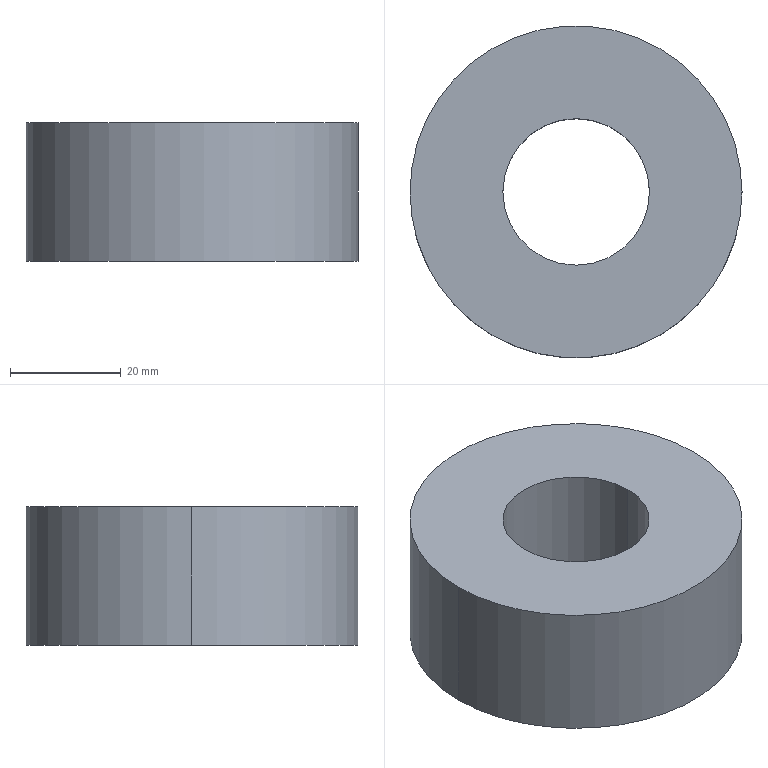Part | SolidWorks | features 3DProfileFeature 1, Extrusion 1, HoleWzd 1 | 1 solid | 6 faces | box 60 x 60 x 25 mm | volume 56897 mm3 | cylinder 4 | plane 2 | commonest cylinder face diameters 26.5 x2 60 x2
STEP:
#1=CARTESIAN_POINT('',(-13.219,-0.003286,0.));
#2=VERTEX_POINT('',#1);
#3=CARTESIAN_POINT('',(13.281,-0.003286,0.));
#4=VERTEX_POINT('',#3);
#5=CARTESIAN_POINT('',(0.03147,-0.003286,0.));
#6=DIRECTION('',(0.,0.,1.));
#7=DIRECTION('',(1.,0.,0.));
#8=AXIS2_PLACEMENT_3D('',#5,#6,#7);
#9=CIRCLE('',#8,13.25);
#10=EDGE_CURVE('',#2,#4,#9,.T.);
#11=ORIENTED_EDGE('',*,*,#10,.F.);
#12=CARTESIAN_POINT('',(-13.219,-0.003286,25.));
#13=VERTEX_POINT('',#12);
#14=CARTESIAN_POINT('',(-13.219,-0.003286,25.));
#15=DIRECTION('',(0.,0.,1.));
#16=VECTOR('',#15,1000.);
#17=LINE('',#14,#16);
#18=EDGE_CURVE('',#2,#13,#17,.T.);
#19=ORIENTED_EDGE('',*,*,#18,.T.);
#20=CARTESIAN_POINT('',(13.281,-0.003286,25.));
#21=VERTEX_POINT('',#20);
#22=CARTESIAN_POINT('',(0.03147,-0.003286,25.));
#23=DIRECTION('',(0.,0.,1.));
#24=DIRECTION('',(1.,0.,0.));
#25=AXIS2_PLACEMENT_3D('',#22,#23,#24);
#26=CIRCLE('',#25,13.25);
#27=EDGE_CURVE('',#13,#21,#26,.T.);
#28=ORIENTED_EDGE('',*,*,#27,.T.);
#29=CARTESIAN_POINT('',(13.281,-0.003286,25.));
#30=DIRECTION('',(0.,0.,1.));
#31=VECTOR('',#30,1000.);
#32=LINE('',#29,#31);
#33=EDGE_CURVE('',#4,#21,#32,.T.);
#34=ORIENTED_EDGE('',*,*,#33,.F.);
#35=EDGE_LOOP('',(#11,#19,#28,#34));
#36=FACE_OUTER_BOUND('',#35,.T.);
#37=CARTESIAN_POINT('',(0.03147,-0.003286,25.));
#38=DIRECTION('',(0.,0.,1.));
#39=DIRECTION('',(1.,0.,0.));
#40=AXIS2_PLACEMENT_3D('',#37,#38,#39);
#41=CYLINDRICAL_SURFACE('',#40,13.25);
#42=ADVANCED_FACE('',(#36),#41,.F.);
#43=CARTESIAN_POINT('',(30.,0.,25.));
#44=VERTEX_POINT('',#43);
#45=CARTESIAN_POINT('',(-30.,0.,25.));
#46=VERTEX_POINT('',#45);
#47=CARTESIAN_POINT('',(0.,0.,25.));
#48=DIRECTION('',(0.,0.,1.));
#49=DIRECTION('',(1.,0.,0.));
#50=AXIS2_PLACEMENT_3D('',#47,#48,#49);
#51=CIRCLE('',#50,30.);
#52=EDGE_CURVE('',#44,#46,#51,.T.);
#53=ORIENTED_EDGE('',*,*,#52,.F.);
#54=CARTESIAN_POINT('',(30.,0.,0.));
#55=VERTEX_POINT('',#54);
#56=CARTESIAN_POINT('',(30.,0.,25.));
#57=DIRECTION('',(0.,0.,-1.));
#58=VECTOR('',#57,1000.);
#59=LINE('',#56,#58);
#60=EDGE_CURVE('',#44,#55,#59,.T.);
#61=ORIENTED_EDGE('',*,*,#60,.T.);
#62=CARTESIAN_POINT('',(-30.,0.,0.));
#63=VERTEX_POINT('',#62);
#64=CARTESIAN_POINT('',(0.,0.,0.));
#65=DIRECTION('',(0.,0.,1.));
#66=DIRECTION('',(1.,0.,0.));
#67=AXIS2_PLACEMENT_3D('',#64,#65,#66);
#68=CIRCLE('',#67,30.);
#69=EDGE_CURVE('',#55,#63,#68,.T.);
#70=ORIENTED_EDGE('',*,*,#69,.T.);
#71=CARTESIAN_POINT('',(-30.,0.,25.));
#72=DIRECTION('',(0.,0.,-1.));
#73=VECTOR('',#72,1000.);
#74=LINE('',#71,#73);
#75=EDGE_CURVE('',#46,#63,#74,.T.);
#76=ORIENTED_EDGE('',*,*,#75,.F.);
#77=EDGE_LOOP('',(#53,#61,#70,#76));
#78=FACE_OUTER_BOUND('',#77,.T.);
#79=CARTESIAN_POINT('',(0.,0.,25.));
#80=DIRECTION('',(0.,0.,-1.));
#81=DIRECTION('',(-1.,0.,0.));
#82=AXIS2_PLACEMENT_3D('',#79,#80,#81);
#83=CYLINDRICAL_SURFACE('',#82,30.);
#84=ADVANCED_FACE('',(#78),#83,.T.);
#85=ORIENTED_EDGE('',*,*,#60,.F.);
#86=CARTESIAN_POINT('',(0.,0.,25.));
#87=DIRECTION('',(0.,0.,1.));
#88=DIRECTION('',(1.,0.,0.));
#89=AXIS2_PLACEMENT_3D('',#86,#87,#88);
#90=CIRCLE('',#89,30.);
#91=EDGE_CURVE('',#46,#44,#90,.T.);
#92=ORIENTED_EDGE('',*,*,#91,.F.);
#93=ORIENTED_EDGE('',*,*,#75,.T.);
#94=CARTESIAN_POINT('',(0.,0.,0.));
#95=DIRECTION('',(0.,0.,1.));
#96=DIRECTION('',(1.,0.,0.));
#97=AXIS2_PLACEMENT_3D('',#94,#95,#96);
#98=CIRCLE('',#97,30.);
#99=EDGE_CURVE('',#63,#55,#98,.T.);
#100=ORIENTED_EDGE('',*,*,#99,.T.);
#101=EDGE_LOOP('',(#85,#92,#93,#100));
#102=FACE_OUTER_BOUND('',#101,.T.);
#103=CARTESIAN_POINT('',(0.,0.,25.));
#104=DIRECTION('',(0.,0.,-1.));
#105=DIRECTION('',(-1.,0.,0.));
#106=AXIS2_PLACEMENT_3D('',#103,#104,#105);
#107=CYLINDRICAL_SURFACE('',#106,30.);
#108=ADVANCED_FACE('',(#102),#107,.T.);
#109=CARTESIAN_POINT('',(0.03147,-0.003286,25.));
#110=DIRECTION('',(0.,0.,1.));
#111=DIRECTION('',(1.,0.,0.));
#112=AXIS2_PLACEMENT_3D('',#109,#110,#111);
#113=CIRCLE('',#112,13.25);
#114=EDGE_CURVE('',#21,#13,#113,.T.);
#115=ORIENTED_EDGE('',*,*,#114,.F.);
#116=ORIENTED_EDGE('',*,*,#27,.F.);
#117=EDGE_LOOP('',(#115,#116));
#118=FACE_BOUND('',#117,.T.);
#119=ORIENTED_EDGE('',*,*,#91,.T.);
#120=ORIENTED_EDGE('',*,*,#52,.T.);
#121=EDGE_LOOP('',(#119,#120));
#122=FACE_OUTER_BOUND('',#121,.T.);
#123=CARTESIAN_POINT('',(0.,0.,25.));
#124=DIRECTION('',(0.,0.,1.));
#125=DIRECTION('',(1.,0.,0.));
#126=AXIS2_PLACEMENT_3D('',#123,#124,#125);
#127=PLANE('',#126);
#128=ADVANCED_FACE('',(#118,#122),#127,.T.);
#129=CARTESIAN_POINT('',(0.03147,-0.003286,0.));
#130=DIRECTION('',(0.,0.,1.));
#131=DIRECTION('',(1.,0.,0.));
#132=AXIS2_PLACEMENT_3D('',#129,#130,#131);
#133=CIRCLE('',#132,13.25);
#134=EDGE_CURVE('',#4,#2,#133,.T.);
#135=ORIENTED_EDGE('',*,*,#134,.T.);
#136=ORIENTED_EDGE('',*,*,#10,.T.);
#137=EDGE_LOOP('',(#135,#136));
#138=FACE_BOUND('',#137,.T.);
#139=ORIENTED_EDGE('',*,*,#99,.F.);
#140=ORIENTED_EDGE('',*,*,#69,.F.);
#141=EDGE_LOOP('',(#139,#140));
#142=FACE_OUTER_BOUND('',#141,.T.);
#143=CARTESIAN_POINT('',(0.,0.,0.));
#144=DIRECTION('',(0.,0.,1.));
#145=DIRECTION('',(1.,0.,0.));
#146=AXIS2_PLACEMENT_3D('',#143,#144,#145);
#147=PLANE('',#146);
#148=ADVANCED_FACE('',(#138,#142),#147,.F.);
#149=ORIENTED_EDGE('',*,*,#18,.F.);
#150=ORIENTED_EDGE('',*,*,#134,.F.);
#151=ORIENTED_EDGE('',*,*,#33,.T.);
#152=ORIENTED_EDGE('',*,*,#114,.T.);
#153=EDGE_LOOP('',(#149,#150,#151,#152));
#154=FACE_OUTER_BOUND('',#153,.T.);
#155=CARTESIAN_POINT('',(0.03147,-0.003286,25.));
#156=DIRECTION('',(0.,0.,1.));
#157=DIRECTION('',(1.,0.,0.));
#158=AXIS2_PLACEMENT_3D('',#155,#156,#157);
#159=CYLINDRICAL_SURFACE('',#158,13.25);
#160=ADVANCED_FACE('',(#154),#159,.F.);
#161=CLOSED_SHELL('',(#42,#84,#108,#128,#148,#160));
#162=MANIFOLD_SOLID_BREP('',#161);
#163=CARTESIAN_POINT('',(0.,0.,0.));
#164=DIRECTION('',(0.,0.,1.));
#165=DIRECTION('',(1.,0.,0.));
#166=AXIS2_PLACEMENT_3D('',#163,#164,#165);
#167=(LENGTH_UNIT()NAMED_UNIT(*)SI_UNIT(.MILLI.,.METRE.));
#168=UNCERTAINTY_MEASURE_WITH_UNIT(LENGTH_MEASURE(0.00001),#167,'','');
#169=(NAMED_UNIT(*)PLANE_ANGLE_UNIT()SI_UNIT($,.RADIAN.));
#170=(NAMED_UNIT(*)SI_UNIT($,.STERADIAN.)SOLID_ANGLE_UNIT());
#171=(GEOMETRIC_REPRESENTATION_CONTEXT(3)GLOBAL_UNCERTAINTY_ASSIGNED_CONTEXT((#168))GLOBAL_UNIT_ASSIGNED_CONTEXT((#167,#169,#170))REPRESENTATION_CONTEXT('',''));
#172=ADVANCED_BREP_SHAPE_REPRESENTATION('',(#162,#166),#171);